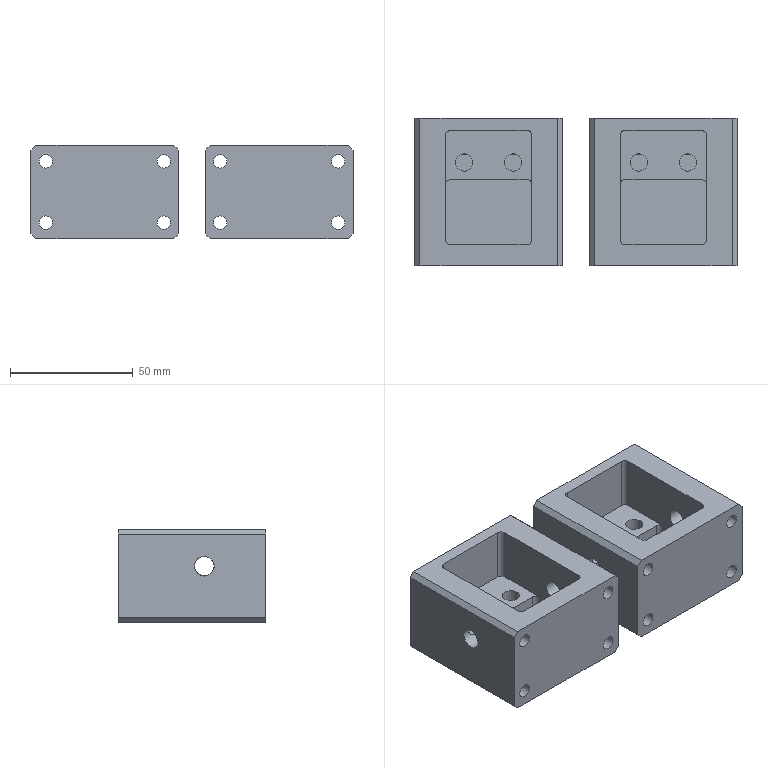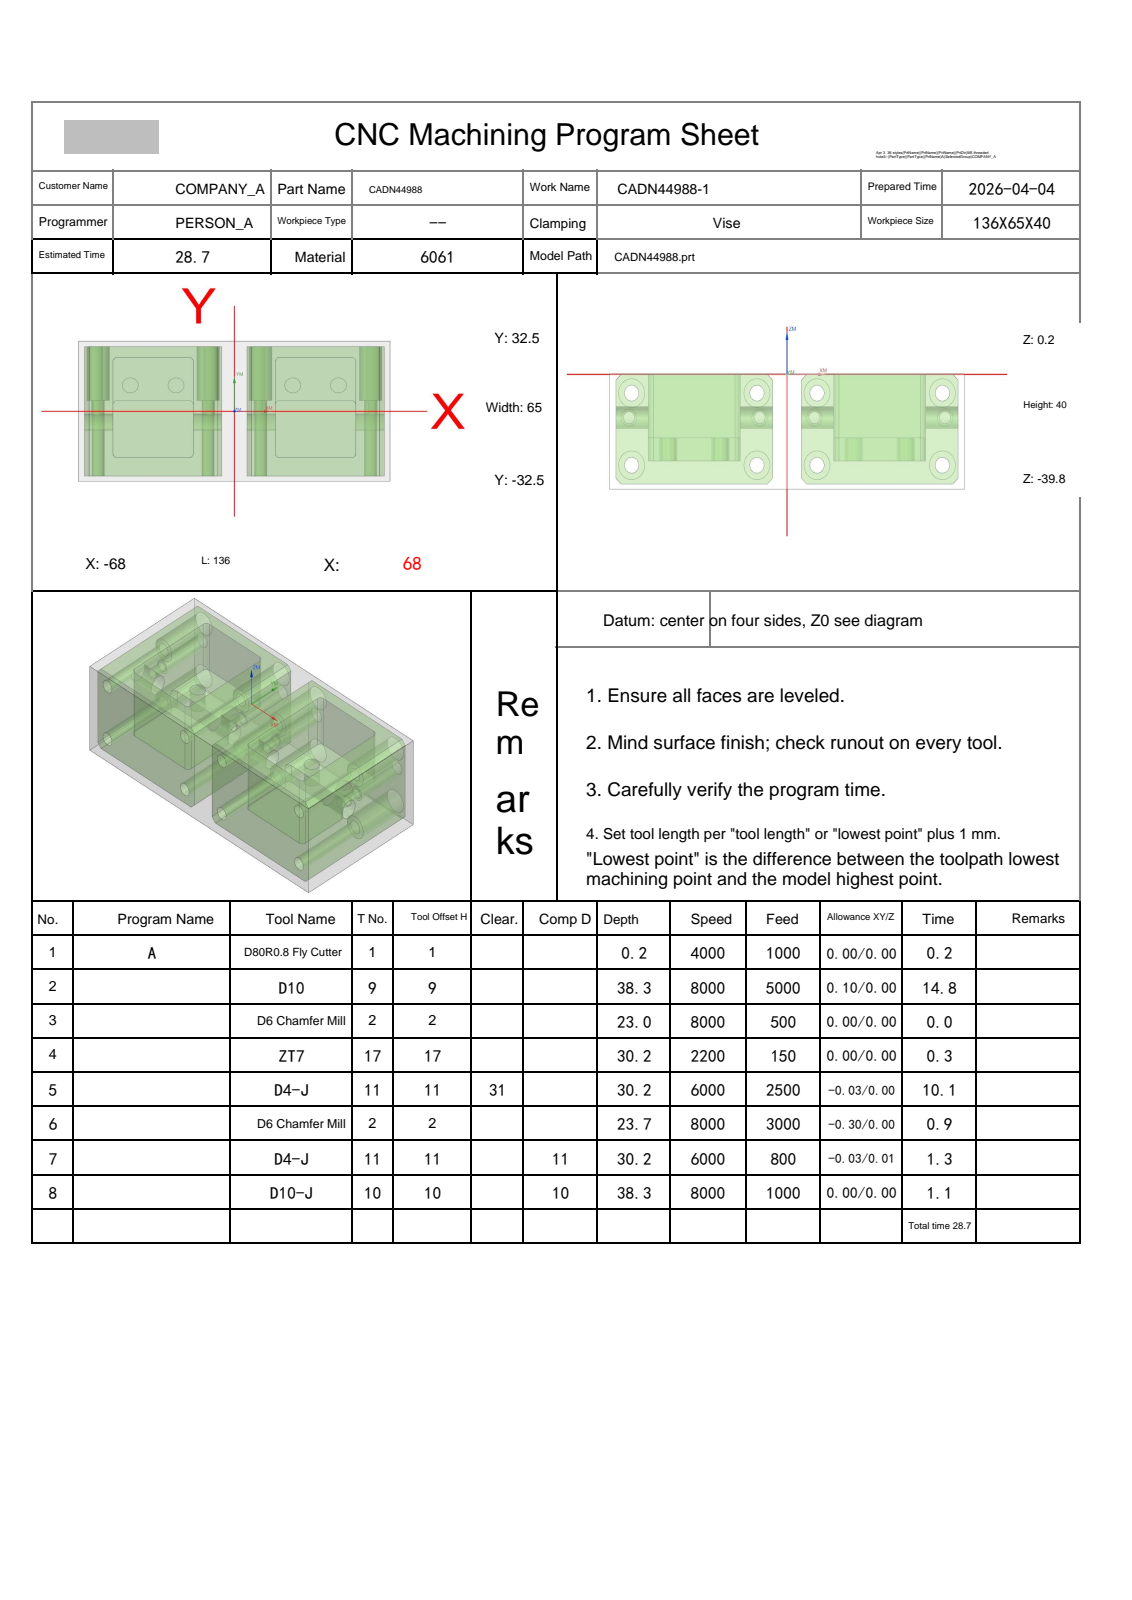NC program | NX | posted by the shop | part box 131 x 60 x 38 mm
Lines 33 to 1162 of 30516:
N2 T09 M06
(D10  D=10. R=0. H=09 ce=0.10 di=0.00)
G00 G90 G54 X35.5 Y-35.1 M03 S8000
G43 H09 Z20.
M08
Z.5
G01 X5.5 Z.413 F5000.
G02 X.4 Y-30. Z.39 I0.0 J5.1
G01 Y30. Z.216
G02 X5.5 Y35.1 Z.193 I5.1 J0.0
G01 X65.5 Z.019
G02 X70.6 Y30. Z-.004 I0.0 J-5.1
G01 Y-30. Z-.178
G02 X65.5 Y-35.1 Z-.201 I-5.1 J0.0
G01 X5.5 Z-.375
G02 X.4 Y-30. Z-.398 I0.0 J5.1
G01 Y30. Z-.572
G02 X5.5 Y35.1 Z-.595 I5.1 J0.0
G01 X65.5 Z-.769
G02 X70.6 Y30. Z-.792 I0.0 J-5.1
G01 Y-30. Z-.965
G02 X65.5 Y-35.1 Z-.989 I-5.1 J0.0
G01 X5.5 Z-1.162
G02 X.4 Y-30. Z-1.186 I0.0 J5.1
G01 Y30. Z-1.359
G02 X5.5 Y35.1 Z-1.383 I5.1 J0.0
G01 X65.5 Z-1.556
G02 X70.6 Y30. Z-1.579 I0.0 J-5.1
G01 Y-30. Z-1.753
G02 X65.5 Y-35.1 Z-1.776 I-5.1 J0.0
G01 X5.5 Z-1.95
G02 X.4 Y-30. Z-1.973 I0.0 J5.1
G01 Y30. Z-2.147
G02 X5.5 Y35.1 Z-2.17 I5.1 J0.0
G01 X65.5 Z-2.344
G02 X70.6 Y30. Z-2.367 I0.0 J-5.1
G01 Y-30. Z-2.541
G02 X65.5 Y-35.1 Z-2.564 I-5.1 J0.0
G01 X5.5 Z-2.738
G02 X.4 Y-30. Z-2.761 I0.0 J5.1
G01 Y30. Z-2.935
G02 X5.5 Y35.1 Z-2.958 I5.1 J0.0
G01 X65.5 Z-3.132
G02 X70.6 Y30. Z-3.155 I0.0 J-5.1
G01 Y-30. Z-3.329
G02 X65.5 Y-35.1 Z-3.352 I-5.1 J0.0
G01 X5.5 Z-3.526
G02 X.4 Y-30. Z-3.549 I0.0 J5.1
G01 Y30. Z-3.723
G02 X5.5 Y35.1 Z-3.746 I5.1 J0.0
G01 X65.5 Z-3.92
G02 X70.6 Y30. Z-3.943 I0.0 J-5.1
G01 Y-30. Z-4.116
G02 X65.5 Y-35.1 Z-4.14 I-5.1 J0.0
G01 X5.5 Z-4.313
G02 X.4 Y-30. Z-4.337 I0.0 J5.1
G01 Y30. Z-4.51
G02 X5.5 Y35.1 Z-4.534 I5.1 J0.0
G01 X65.5 Z-4.707
G02 X70.6 Y30. Z-4.73 I0.0 J-5.1
G01 Y-30. Z-4.904
G02 X65.5 Y-35.1 Z-4.927 I-5.1 J0.0
G01 X5.5 Z-5.101
G02 X.4 Y-30. Z-5.124 I0.0 J5.1
G01 Y30. Z-5.298
G02 X5.5 Y35.1 Z-5.321 I5.1 J0.0
G01 X65.5 Z-5.495
G02 X70.6 Y30. Z-5.518 I0.0 J-5.1
G01 Y-30. Z-5.692
G02 X65.5 Y-35.1 Z-5.715 I-5.1 J0.0
G01 X5.5 Z-5.889
G02 X.4 Y-30. Z-5.912 I0.0 J5.1
G01 Y30. Z-6.086
G02 X5.5 Y35.1 Z-6.109 I5.1 J0.0
G01 X65.5 Z-6.283
G02 X70.6 Y30. Z-6.306 I0.0 J-5.1
G01 Y-30. Z-6.48
G02 X65.5 Y-35.1 Z-6.503 I-5.1 J0.0
G01 X5.5 Z-6.677
G02 X.4 Y-30. Z-6.7 I0.0 J5.1
G01 Y30. Z-6.874
G02 X5.5 Y35.1 Z-6.897 I5.1 J0.0
G01 X65.5 Z-7.071
G02 X70.6 Y30. Z-7.094 I0.0 J-5.1
G01 Y-30. Z-7.267
G02 X65.5 Y-35.1 Z-7.291 I-5.1 J0.0
G01 X5.5 Z-7.464
G02 X.4 Y-30. Z-7.488 I0.0 J5.1
G01 Y30. Z-7.661
G02 X5.5 Y35.1 Z-7.685 I5.1 J0.0
G01 X65.5 Z-7.858
G02 X70.6 Y30. Z-7.881 I0.0 J-5.1
G01 Y-30. Z-8.055
G02 X65.5 Y-35.1 Z-8.078 I-5.1 J0.0
G01 X5.5 Z-8.252
G02 X.4 Y-30. Z-8.275 I0.0 J5.1
G01 Y30. Z-8.449
G02 X5.5 Y35.1 Z-8.472 I5.1 J0.0
G01 X65.5 Z-8.646
G02 X70.6 Y30. Z-8.669 I0.0 J-5.1
G01 Y-30. Z-8.843
G02 X65.5 Y-35.1 Z-8.866 I-5.1 J0.0
G01 X5.5 Z-9.04
G02 X.4 Y-30. Z-9.063 I0.0 J5.1
G01 Y30. Z-9.237
G02 X5.5 Y35.1 Z-9.26 I5.1 J0.0
G01 X65.5 Z-9.434
G02 X70.6 Y30. Z-9.457 I0.0 J-5.1
G01 Y-30. Z-9.631
G02 X65.5 Y-35.1 Z-9.654 I-5.1 J0.0
G01 X5.5 Z-9.828
G02 X.4 Y-30. Z-9.851 I0.0 J5.1
G01 Y30. Z-10.025
G02 X5.5 Y35.1 Z-10.048 I5.1 J0.0
G01 X65.5 Z-10.222
G02 X70.6 Y30. Z-10.245 I0.0 J-5.1
G01 Y-30. Z-10.419
G02 X65.5 Y-35.1 Z-10.442 I-5.1 J0.0
G01 X5.5 Z-10.615
G02 X.4 Y-30. Z-10.639 I0.0 J5.1
G01 Y30. Z-10.812
G02 X5.5 Y35.1 Z-10.836 I5.1 J0.0
G01 X65.5 Z-11.009
G02 X70.6 Y30. Z-11.033 I0.0 J-5.1
G01 Y-30. Z-11.206
G02 X65.5 Y-35.1 Z-11.229 I-5.1 J0.0
G01 X5.5 Z-11.403
G02 X.4 Y-30. Z-11.426 I0.0 J5.1
G01 Y30. Z-11.6
G02 X5.5 Y35.1 Z-11.623 I5.1 J0.0
G01 X65.5 Z-11.797
G02 X70.6 Y30. Z-11.82 I0.0 J-5.1
G01 Y-30. Z-11.994
G02 X65.5 Y-35.1 Z-12.017 I-5.1 J0.0
G01 X5.5 Z-12.191
G02 X.4 Y-30. Z-12.214 I0.0 J5.1
G01 Y30. Z-12.388
G02 X5.5 Y35.1 Z-12.411 I5.1 J0.0
G01 X65.5 Z-12.585
G02 X70.6 Y30. Z-12.608 I0.0 J-5.1
G01 Y-30. Z-12.782
G02 X65.5 Y-35.1 Z-12.805 I-5.1 J0.0
G01 X5.5 Z-12.979
G02 X.4 Y-30. Z-13.002 I0.0 J5.1
G01 Y30. Z-13.176
G02 X5.5 Y35.1 Z-13.199 I5.1 J0.0
G01 X65.5 Z-13.373
G02 X70.6 Y30. Z-13.396 I0.0 J-5.1
G01 Y-30. Z-13.57
G02 X65.5 Y-35.1 Z-13.593 I-5.1 J0.0
G01 X5.5 Z-13.766
G02 X.4 Y-30. Z-13.79 I0.0 J5.1
G01 Y30. Z-13.963
G02 X5.5 Y35.1 Z-13.987 I5.1 J0.0
G01 X65.5 Z-14.16
G02 X70.6 Y30. Z-14.184 I0.0 J-5.1
G01 Y-30. Z-14.357
G02 X65.5 Y-35.1 Z-14.38 I-5.1 J0.0
G01 X5.5 Z-14.554
G02 X.4 Y-30. Z-14.577 I0.0 J5.1
G01 Y30. Z-14.751
G02 X5.5 Y35.1 Z-14.774 I5.1 J0.0
G01 X65.5 Z-14.948
G02 X70.6 Y30. Z-14.971 I0.0 J-5.1
G01 Y-30. Z-15.145
G02 X65.5 Y-35.1 Z-15.168 I-5.1 J0.0
G01 X5.5 Z-15.342
G02 X.4 Y-30. Z-15.365 I0.0 J5.1
G01 Y30. Z-15.539
G02 X5.5 Y35.1 Z-15.562 I5.1 J0.0
G01 X65.5 Z-15.736
G02 X70.6 Y30. Z-15.759 I0.0 J-5.1
G01 Y-30. Z-15.933
G02 X65.5 Y-35.1 Z-15.956 I-5.1 J0.0
G01 X5.5 Z-16.13
G02 X.4 Y-30. Z-16.153 I0.0 J5.1
G01 Y30. Z-16.327
G02 X5.5 Y35.1 Z-16.35 I5.1 J0.0
G01 X65.5 Z-16.524
G02 X70.6 Y30. Z-16.547 I0.0 J-5.1
G01 Y-30. Z-16.721
G02 X65.5 Y-35.1 Z-16.744 I-5.1 J0.0
G01 X5.5 Z-16.917
G02 X.4 Y-30. Z-16.941 I0.0 J5.1
G01 Y30. Z-17.114
G02 X5.5 Y35.1 Z-17.138 I5.1 J0.0
G01 X65.5 Z-17.311
G02 X70.6 Y30. Z-17.335 I0.0 J-5.1
G01 Y-30. Z-17.508
G02 X65.5 Y-35.1 Z-17.531 I-5.1 J0.0
G01 X5.5 Z-17.705
G02 X.4 Y-30. Z-17.728 I0.0 J5.1
G01 Y30. Z-17.902
G02 X5.5 Y35.1 Z-17.925 I5.1 J0.0
G01 X65.5 Z-18.099
G02 X70.6 Y30. Z-18.122 I0.0 J-5.1
G01 Y-30. Z-18.296
G02 X65.5 Y-35.1 Z-18.319 I-5.1 J0.0
G01 X5.5 Z-18.493
G02 X.4 Y-30. Z-18.516 I0.0 J5.1
G01 Y30. Z-18.69
G02 X5.5 Y35.1 Z-18.713 I5.1 J0.0
G01 X65.5 Z-18.887
G02 X70.6 Y30. Z-18.91 I0.0 J-5.1
G01 Y-30. Z-19.084
G02 X65.5 Y-35.1 Z-19.107 I-5.1 J0.0
G01 X5.5 Z-19.281
G02 X.4 Y-30. Z-19.304 I0.0 J5.1
G01 Y30. Z-19.478
G02 X5.5 Y35.1 Z-19.501 I5.1 J0.0
G01 X65.5 Z-19.675
G02 X70.6 Y30. Z-19.698 I0.0 J-5.1
G01 Y-30. Z-19.872
G02 X65.5 Y-35.1 Z-19.895 I-5.1 J0.0
G01 X5.5 Z-20.069
G02 X.4 Y-30. Z-20.092 I0.0 J5.1
G01 Y30. Z-20.265
G02 X5.5 Y35.1 Z-20.289 I5.1 J0.0
G01 X65.5 Z-20.462
G02 X70.6 Y30. Z-20.486 I0.0 J-5.1
G01 Y-30. Z-20.659
G02 X65.5 Y-35.1 Z-20.683 I-5.1 J0.0
G01 X5.5 Z-20.856
G02 X.4 Y-30. Z-20.879 I0.0 J5.1
G01 Y30. Z-21.053
G02 X5.5 Y35.1 Z-21.076 I5.1 J0.0
G01 X65.5 Z-21.25
G02 X70.6 Y30. Z-21.273 I0.0 J-5.1
G01 Y-30. Z-21.447
G02 X65.5 Y-35.1 Z-21.47 I-5.1 J0.0
G01 X5.5 Z-21.644
G02 X.4 Y-30. Z-21.667 I0.0 J5.1
G01 Y30. Z-21.841
G02 X5.5 Y35.1 Z-21.864 I5.1 J0.0
G01 X65.5 Z-22.038
G02 X70.6 Y30. Z-22.061 I0.0 J-5.1
G01 Y-30. Z-22.235
G02 X65.5 Y-35.1 Z-22.258 I-5.1 J0.0
G01 X5.5 Z-22.432
G02 X.4 Y-30. Z-22.455 I0.0 J5.1
G01 Y30. Z-22.629
G02 X5.5 Y35.1 Z-22.652 I5.1 J0.0
G01 X65.5 Z-22.826
G02 X70.6 Y30. Z-22.849 I0.0 J-5.1
G01 Y-30. Z-23.023
G02 X65.5 Y-35.1 Z-23.046 I-5.1 J0.0
G01 X5.5 Z-23.22
G02 X.4 Y-30. Z-23.243 I0.0 J5.1
G01 Y30. Z-23.416
G02 X5.5 Y35.1 Z-23.44 I5.1 J0.0
G01 X65.5 Z-23.613
G02 X70.6 Y30. Z-23.637 I0.0 J-5.1
G01 Y-30. Z-23.81
G02 X65.5 Y-35.1 Z-23.834 I-5.1 J0.0
G01 X5.5 Z-24.007
G02 X.4 Y-30. Z-24.03 I0.0 J5.1
G01 Y30. Z-24.204
G02 X5.5 Y35.1 Z-24.227 I5.1 J0.0
G01 X65.5 Z-24.401
G02 X70.6 Y30. Z-24.424 I0.0 J-5.1
G01 Y-30. Z-24.598
G02 X65.5 Y-35.1 Z-24.621 I-5.1 J0.0
G01 X5.5 Z-24.795
G02 X.4 Y-30. Z-24.818 I0.0 J5.1
G01 Y30. Z-24.992
G02 X5.5 Y35.1 Z-25.015 I5.1 J0.0
G01 X65.5 Z-25.189
G02 X70.6 Y30. Z-25.212 I0.0 J-5.1
G01 Y-30. Z-25.386
G02 X65.5 Y-35.1 Z-25.409 I-5.1 J0.0
G01 X5.5 Z-25.583
G02 X.4 Y-30. Z-25.606 I0.0 J5.1
G01 Y30. Z-25.78
G02 X5.5 Y35.1 Z-25.803 I5.1 J0.0
G01 X65.5 Z-25.977
G02 X70.6 Y30. Z-26. I0.0 J-5.1
G01 Y-30. Z-26.174
G02 X65.5 Y-35.1 Z-26.197 I-5.1 J0.0
G01 X5.5 Z-26.371
G02 X.4 Y-30. Z-26.394 I0.0 J5.1
G01 Y30. Z-26.567
G02 X5.5 Y35.1 Z-26.591 I5.1 J0.0
G01 X65.5 Z-26.764
G02 X70.6 Y30. Z-26.788 I0.0 J-5.1
G01 Y-30. Z-26.961
G02 X65.5 Y-35.1 Z-26.985 I-5.1 J0.0
G01 X5.5 Z-27.158
G02 X.4 Y-30. Z-27.181 I0.0 J5.1
G01 Y30. Z-27.355
G02 X5.5 Y35.1 Z-27.378 I5.1 J0.0
G01 X65.5 Z-27.552
G02 X70.6 Y30. Z-27.575 I0.0 J-5.1
G01 Y-30. Z-27.749
G02 X65.5 Y-35.1 Z-27.772 I-5.1 J0.0
G01 X5.5 Z-27.946
G02 X.4 Y-30. Z-27.969 I0.0 J5.1
G01 Y30. Z-28.143
G02 X5.5 Y35.1 Z-28.166 I5.1 J0.0
G01 X65.5 Z-28.34
G02 X70.6 Y30. Z-28.363 I0.0 J-5.1
G01 Y-30. Z-28.537
G02 X65.5 Y-35.1 Z-28.56 I-5.1 J0.0
G01 X5.5 Z-28.734
G02 X.4 Y-30. Z-28.757 I0.0 J5.1
G01 Y30. Z-28.931
G02 X5.5 Y35.1 Z-28.954 I5.1 J0.0
G01 X65.5 Z-29.128
G02 X70.6 Y30. Z-29.151 I0.0 J-5.1
G01 Y-30. Z-29.325
G02 X65.5 Y-35.1 Z-29.348 I-5.1 J0.0
G01 X5.5 Z-29.522
G02 X.4 Y-30. Z-29.545 I0.0 J5.1
G01 Y30. Z-29.719
G02 X5.5 Y35.1 Z-29.742 I5.1 J0.0
G01 X65.5 Z-29.915
G02 X70.6 Y30. Z-29.939 I0.0 J-5.1
G01 Y-30. Z-30.112
G02 X65.5 Y-35.1 Z-30.136 I-5.1 J0.0
G01 X5.5 Z-30.309
G02 X.4 Y-30. Z-30.333 I0.0 J5.1
G01 Y30. Z-30.506
G02 X5.5 Y35.1 Z-30.529 I5.1 J0.0
G01 X65.5 Z-30.703
G02 X70.6 Y30. Z-30.726 I0.0 J-5.1
G01 Y-30. Z-30.9
G02 X65.5 Y-35.1 Z-30.923 I-5.1 J0.0
G01 X5.5 Z-31.097
G02 X.4 Y-30. Z-31.12 I0.0 J5.1
G01 Y30. Z-31.294
G02 X5.5 Y35.1 Z-31.317 I5.1 J0.0
G01 X65.5 Z-31.491
G02 X70.6 Y30. Z-31.514 I0.0 J-5.1
G01 Y-30. Z-31.688
G02 X65.5 Y-35.1 Z-31.711 I-5.1 J0.0
G01 X5.5 Z-31.885
G02 X.4 Y-30. Z-31.908 I0.0 J5.1
G01 Y30. Z-32.082
G02 X5.5 Y35.1 Z-32.105 I5.1 J0.0
G01 X65.5 Z-32.279
G02 X70.6 Y30. Z-32.302 I0.0 J-5.1
G01 Y-30. Z-32.476
G02 X65.5 Y-35.1 Z-32.499 I-5.1 J0.0
G01 X5.5 Z-32.673
G02 X.4 Y-30. Z-32.696 I0.0 J5.1
G01 Y30. Z-32.87
G02 X5.5 Y35.1 Z-32.893 I5.1 J0.0
G01 X65.5 Z-33.066
G02 X70.6 Y30. Z-33.09 I0.0 J-5.1
G01 Y-30. Z-33.263
G02 X65.5 Y-35.1 Z-33.287 I-5.1 J0.0
G01 X5.5 Z-33.46
G02 X.4 Y-30. Z-33.484 I0.0 J5.1
G01 Y30. Z-33.657
G02 X5.5 Y35.1 Z-33.68 I5.1 J0.0
G01 X65.5 Z-33.854
G02 X70.6 Y30. Z-33.877 I0.0 J-5.1
G01 Y-30. Z-34.051
G02 X65.5 Y-35.1 Z-34.074 I-5.1 J0.0
G01 X5.5 Z-34.248
G02 X.4 Y-30. Z-34.271 I0.0 J5.1
G01 Y30. Z-34.445
G02 X5.5 Y35.1 Z-34.468 I5.1 J0.0
G01 X65.5 Z-34.642
G02 X70.6 Y30. Z-34.665 I0.0 J-5.1
G01 Y-30. Z-34.839
G02 X65.5 Y-35.1 Z-34.862 I-5.1 J0.0
G01 X5.5 Z-35.036
G02 X.4 Y-30. Z-35.059 I0.0 J5.1
G01 Y30. Z-35.233
G02 X5.5 Y35.1 Z-35.256 I5.1 J0.0
G01 X65.5 Z-35.43
G02 X70.6 Y30. Z-35.453 I0.0 J-5.1
G01 Y-30. Z-35.627
G02 X65.5 Y-35.1 Z-35.65 I-5.1 J0.0
G01 X5.5 Z-35.824
G02 X.4 Y-30. Z-35.847 I0.0 J5.1
G01 Y30. Z-36.021
G02 X5.5 Y35.1 Z-36.044 I5.1 J0.0
G01 X65.5 Z-36.217
G02 X70.6 Y30. Z-36.241 I0.0 J-5.1
G01 Y-30. Z-36.414
G02 X65.5 Y-35.1 Z-36.438 I-5.1 J0.0
G01 X5.5 Z-36.611
G02 X.4 Y-30. Z-36.635 I0.0 J5.1
G01 Y30. Z-36.808
G02 X5.5 Y35.1 Z-36.831 I5.1 J0.0
G01 X65.5 Z-37.005
G02 X70.6 Y30. Z-37.028 I0.0 J-5.1
G01 Y-30. Z-37.202
G02 X65.5 Y-35.1 Z-37.225 I-5.1 J0.0
G01 X5.5 Z-37.399
G02 X.4 Y-30. Z-37.422 I0.0 J5.1
G01 Y30. Z-37.596
G02 X5.5 Y35.1 Z-37.619 I5.1 J0.0
G01 X65.5 Z-37.793
G02 X70.6 Y30. Z-37.816 I0.0 J-5.1
G01 Y-30. Z-37.99
G02 X65.5 Y-35.1 Z-38.013 I-5.1 J0.0
G01 X35.5 Z-38.1
X5.5
G02 X.4 Y-30. I0.0 J5.1
G01 Y30.
G02 X5.5 Y35.1 I5.1 J0.0
G01 X65.5
G02 X70.6 Y30. I0.0 J-5.1
G01 Y-30.
G02 X65.5 Y-35.1 I-5.1 J0.0
G01 X35.5
X35.
Z-37.1
G00 Z20.
X-35.5
Z.5
G01 X-65.5 Z.413
G02 X-70.6 Y-30. Z.39 I0.0 J5.1
G01 Y30. Z.216
G02 X-65.5 Y35.1 Z.193 I5.1 J0.0
G01 X-5.5 Z.019
G02 X-.4 Y30. Z-.004 I0.0 J-5.1
G01 Y-30. Z-.178
G02 X-5.5 Y-35.1 Z-.201 I-5.1 J0.0
G01 X-65.5 Z-.375
G02 X-70.6 Y-30. Z-.398 I0.0 J5.1
G01 Y30. Z-.572
G02 X-65.5 Y35.1 Z-.595 I5.1 J0.0
G01 X-5.5 Z-.769
G02 X-.4 Y30. Z-.792 I0.0 J-5.1
G01 Y-30. Z-.965
G02 X-5.5 Y-35.1 Z-.989 I-5.1 J0.0
G01 X-65.5 Z-1.162
G02 X-70.6 Y-30. Z-1.186 I0.0 J5.1
G01 Y30. Z-1.359
G02 X-65.5 Y35.1 Z-1.383 I5.1 J0.0
G01 X-5.5 Z-1.556
G02 X-.4 Y30. Z-1.579 I0.0 J-5.1
G01 Y-30. Z-1.753
G02 X-5.5 Y-35.1 Z-1.776 I-5.1 J0.0
G01 X-65.5 Z-1.95
G02 X-70.6 Y-30. Z-1.973 I0.0 J5.1
G01 Y30. Z-2.147
G02 X-65.5 Y35.1 Z-2.17 I5.1 J0.0
G01 X-5.5 Z-2.344
G02 X-.4 Y30. Z-2.367 I0.0 J-5.1
G01 Y-30. Z-2.541
G02 X-5.5 Y-35.1 Z-2.564 I-5.1 J0.0
G01 X-65.5 Z-2.738
G02 X-70.6 Y-30. Z-2.761 I0.0 J5.1
G01 Y30. Z-2.935
G02 X-65.5 Y35.1 Z-2.958 I5.1 J0.0
G01 X-5.5 Z-3.132
G02 X-.4 Y30. Z-3.155 I0.0 J-5.1
G01 Y-30. Z-3.329
G02 X-5.5 Y-35.1 Z-3.352 I-5.1 J0.0
G01 X-65.5 Z-3.526
G02 X-70.6 Y-30. Z-3.549 I0.0 J5.1
G01 Y30. Z-3.723
G02 X-65.5 Y35.1 Z-3.746 I5.1 J0.0
G01 X-5.5 Z-3.92
G02 X-.4 Y30. Z-3.943 I0.0 J-5.1
G01 Y-30. Z-4.116
G02 X-5.5 Y-35.1 Z-4.14 I-5.1 J0.0
G01 X-65.5 Z-4.313
G02 X-70.6 Y-30. Z-4.337 I0.0 J5.1
G01 Y30. Z-4.51
G02 X-65.5 Y35.1 Z-4.534 I5.1 J0.0
G01 X-5.5 Z-4.707
G02 X-.4 Y30. Z-4.73 I0.0 J-5.1
G01 Y-30. Z-4.904
G02 X-5.5 Y-35.1 Z-4.927 I-5.1 J0.0
G01 X-65.5 Z-5.101
G02 X-70.6 Y-30. Z-5.124 I0.0 J5.1
G01 Y30. Z-5.298
G02 X-65.5 Y35.1 Z-5.321 I5.1 J0.0
G01 X-5.5 Z-5.495
G02 X-.4 Y30. Z-5.518 I0.0 J-5.1
G01 Y-30. Z-5.692
G02 X-5.5 Y-35.1 Z-5.715 I-5.1 J0.0
G01 X-65.5 Z-5.889
G02 X-70.6 Y-30. Z-5.912 I0.0 J5.1
G01 Y30. Z-6.086
G02 X-65.5 Y35.1 Z-6.109 I5.1 J0.0
G01 X-5.5 Z-6.283
G02 X-.4 Y30. Z-6.306 I0.0 J-5.1
G01 Y-30. Z-6.48
G02 X-5.5 Y-35.1 Z-6.503 I-5.1 J0.0
G01 X-65.5 Z-6.677
G02 X-70.6 Y-30. Z-6.7 I0.0 J5.1
G01 Y30. Z-6.874
G02 X-65.5 Y35.1 Z-6.897 I5.1 J0.0
G01 X-5.5 Z-7.071
G02 X-.4 Y30. Z-7.094 I0.0 J-5.1
G01 Y-30. Z-7.267
G02 X-5.5 Y-35.1 Z-7.291 I-5.1 J0.0
G01 X-65.5 Z-7.464
G02 X-70.6 Y-30. Z-7.488 I0.0 J5.1
G01 Y30. Z-7.661
G02 X-65.5 Y35.1 Z-7.685 I5.1 J0.0
G01 X-5.5 Z-7.858
G02 X-.4 Y30. Z-7.881 I0.0 J-5.1
G01 Y-30. Z-8.055
G02 X-5.5 Y-35.1 Z-8.078 I-5.1 J0.0
G01 X-65.5 Z-8.252
G02 X-70.6 Y-30. Z-8.275 I0.0 J5.1
G01 Y30. Z-8.449
G02 X-65.5 Y35.1 Z-8.472 I5.1 J0.0
G01 X-5.5 Z-8.646
G02 X-.4 Y30. Z-8.669 I0.0 J-5.1
G01 Y-30. Z-8.843
G02 X-5.5 Y-35.1 Z-8.866 I-5.1 J0.0
G01 X-65.5 Z-9.04
G02 X-70.6 Y-30. Z-9.063 I0.0 J5.1
G01 Y30. Z-9.237
G02 X-65.5 Y35.1 Z-9.26 I5.1 J0.0
G01 X-5.5 Z-9.434
G02 X-.4 Y30. Z-9.457 I0.0 J-5.1
G01 Y-30. Z-9.631
G02 X-5.5 Y-35.1 Z-9.654 I-5.1 J0.0
G01 X-65.5 Z-9.828
G02 X-70.6 Y-30. Z-9.851 I0.0 J5.1
G01 Y30. Z-10.025
G02 X-65.5 Y35.1 Z-10.048 I5.1 J0.0
G01 X-5.5 Z-10.222
G02 X-.4 Y30. Z-10.245 I0.0 J-5.1
G01 Y-30. Z-10.419
G02 X-5.5 Y-35.1 Z-10.442 I-5.1 J0.0
G01 X-65.5 Z-10.615
G02 X-70.6 Y-30. Z-10.639 I0.0 J5.1
G01 Y30. Z-10.812
G02 X-65.5 Y35.1 Z-10.836 I5.1 J0.0
G01 X-5.5 Z-11.009
G02 X-.4 Y30. Z-11.033 I0.0 J-5.1
G01 Y-30. Z-11.206
G02 X-5.5 Y-35.1 Z-11.229 I-5.1 J0.0
G01 X-65.5 Z-11.403
G02 X-70.6 Y-30. Z-11.426 I0.0 J5.1
G01 Y30. Z-11.6
G02 X-65.5 Y35.1 Z-11.623 I5.1 J0.0
G01 X-5.5 Z-11.797
G02 X-.4 Y30. Z-11.82 I0.0 J-5.1
G01 Y-30. Z-11.994
G02 X-5.5 Y-35.1 Z-12.017 I-5.1 J0.0
G01 X-65.5 Z-12.191
G02 X-70.6 Y-30. Z-12.214 I0.0 J5.1
G01 Y30. Z-12.388
G02 X-65.5 Y35.1 Z-12.411 I5.1 J0.0
G01 X-5.5 Z-12.585
G02 X-.4 Y30. Z-12.608 I0.0 J-5.1
G01 Y-30. Z-12.782
G02 X-5.5 Y-35.1 Z-12.805 I-5.1 J0.0
G01 X-65.5 Z-12.979
G02 X-70.6 Y-30. Z-13.002 I0.0 J5.1
G01 Y30. Z-13.176
G02 X-65.5 Y35.1 Z-13.199 I5.1 J0.0
G01 X-5.5 Z-13.373
G02 X-.4 Y30. Z-13.396 I0.0 J-5.1
G01 Y-30. Z-13.57
G02 X-5.5 Y-35.1 Z-13.593 I-5.1 J0.0
G01 X-65.5 Z-13.766
G02 X-70.6 Y-30. Z-13.79 I0.0 J5.1
G01 Y30. Z-13.963
G02 X-65.5 Y35.1 Z-13.987 I5.1 J0.0
G01 X-5.5 Z-14.16
G02 X-.4 Y30. Z-14.184 I0.0 J-5.1
G01 Y-30. Z-14.357
G02 X-5.5 Y-35.1 Z-14.38 I-5.1 J0.0
G01 X-65.5 Z-14.554
G02 X-70.6 Y-30. Z-14.577 I0.0 J5.1
G01 Y30. Z-14.751
G02 X-65.5 Y35.1 Z-14.774 I5.1 J0.0
G01 X-5.5 Z-14.948
G02 X-.4 Y30. Z-14.971 I0.0 J-5.1
G01 Y-30. Z-15.145
G02 X-5.5 Y-35.1 Z-15.168 I-5.1 J0.0
G01 X-65.5 Z-15.342
G02 X-70.6 Y-30. Z-15.365 I0.0 J5.1
G01 Y30. Z-15.539
G02 X-65.5 Y35.1 Z-15.562 I5.1 J0.0
G01 X-5.5 Z-15.736
G02 X-.4 Y30. Z-15.759 I0.0 J-5.1
G01 Y-30. Z-15.933
G02 X-5.5 Y-35.1 Z-15.956 I-5.1 J0.0
G01 X-65.5 Z-16.13
G02 X-70.6 Y-30. Z-16.153 I0.0 J5.1
G01 Y30. Z-16.327
G02 X-65.5 Y35.1 Z-16.35 I5.1 J0.0
G01 X-5.5 Z-16.524
G02 X-.4 Y30. Z-16.547 I0.0 J-5.1
G01 Y-30. Z-16.721
G02 X-5.5 Y-35.1 Z-16.744 I-5.1 J0.0
G01 X-65.5 Z-16.917
G02 X-70.6 Y-30. Z-16.941 I0.0 J5.1
G01 Y30. Z-17.114
G02 X-65.5 Y35.1 Z-17.138 I5.1 J0.0
G01 X-5.5 Z-17.311
G02 X-.4 Y30. Z-17.335 I0.0 J-5.1
G01 Y-30. Z-17.508
G02 X-5.5 Y-35.1 Z-17.531 I-5.1 J0.0
G01 X-65.5 Z-17.705
G02 X-70.6 Y-30. Z-17.728 I0.0 J5.1
G01 Y30. Z-17.902
G02 X-65.5 Y35.1 Z-17.925 I5.1 J0.0
G01 X-5.5 Z-18.099
G02 X-.4 Y30. Z-18.122 I0.0 J-5.1
G01 Y-30. Z-18.296
G02 X-5.5 Y-35.1 Z-18.319 I-5.1 J0.0
G01 X-65.5 Z-18.493
G02 X-70.6 Y-30. Z-18.516 I0.0 J5.1
G01 Y30. Z-18.69
G02 X-65.5 Y35.1 Z-18.713 I5.1 J0.0
G01 X-5.5 Z-18.887
G02 X-.4 Y30. Z-18.91 I0.0 J-5.1
G01 Y-30. Z-19.084
G02 X-5.5 Y-35.1 Z-19.107 I-5.1 J0.0
G01 X-65.5 Z-19.281
G02 X-70.6 Y-30. Z-19.304 I0.0 J5.1
G01 Y30. Z-19.478
G02 X-65.5 Y35.1 Z-19.501 I5.1 J0.0
G01 X-5.5 Z-19.675
G02 X-.4 Y30. Z-19.698 I0.0 J-5.1
G01 Y-30. Z-19.872
G02 X-5.5 Y-35.1 Z-19.895 I-5.1 J0.0
G01 X-65.5 Z-20.069
G02 X-70.6 Y-30. Z-20.092 I0.0 J5.1
G01 Y30. Z-20.265
G02 X-65.5 Y35.1 Z-20.289 I5.1 J0.0
G01 X-5.5 Z-20.462
G02 X-.4 Y30. Z-20.486 I0.0 J-5.1
G01 Y-30. Z-20.659
G02 X-5.5 Y-35.1 Z-20.683 I-5.1 J0.0
G01 X-65.5 Z-20.856
G02 X-70.6 Y-30. Z-20.879 I0.0 J5.1
G01 Y30. Z-21.053
G02 X-65.5 Y35.1 Z-21.076 I5.1 J0.0
G01 X-5.5 Z-21.25
G02 X-.4 Y30. Z-21.273 I0.0 J-5.1
G01 Y-30. Z-21.447
G02 X-5.5 Y-35.1 Z-21.47 I-5.1 J0.0
G01 X-65.5 Z-21.644
G02 X-70.6 Y-30. Z-21.667 I0.0 J5.1
G01 Y30. Z-21.841
G02 X-65.5 Y35.1 Z-21.864 I5.1 J0.0
G01 X-5.5 Z-22.038
G02 X-.4 Y30. Z-22.061 I0.0 J-5.1
G01 Y-30. Z-22.235
G02 X-5.5 Y-35.1 Z-22.258 I-5.1 J0.0
G01 X-65.5 Z-22.432
G02 X-70.6 Y-30. Z-22.455 I0.0 J5.1
G01 Y30. Z-22.629
G02 X-65.5 Y35.1 Z-22.652 I5.1 J0.0
G01 X-5.5 Z-22.826
G02 X-.4 Y30. Z-22.849 I0.0 J-5.1
G01 Y-30. Z-23.023
G02 X-5.5 Y-35.1 Z-23.046 I-5.1 J0.0
G01 X-65.5 Z-23.22
G02 X-70.6 Y-30. Z-23.243 I0.0 J5.1
G01 Y30. Z-23.416
G02 X-65.5 Y35.1 Z-23.44 I5.1 J0.0
G01 X-5.5 Z-23.613
G02 X-.4 Y30. Z-23.637 I0.0 J-5.1
G01 Y-30. Z-23.81
G02 X-5.5 Y-35.1 Z-23.834 I-5.1 J0.0
G01 X-65.5 Z-24.007
G02 X-70.6 Y-30. Z-24.03 I0.0 J5.1
G01 Y30. Z-24.204
G02 X-65.5 Y35.1 Z-24.227 I5.1 J0.0
G01 X-5.5 Z-24.401
G02 X-.4 Y30. Z-24.424 I0.0 J-5.1
G01 Y-30. Z-24.598
G02 X-5.5 Y-35.1 Z-24.621 I-5.1 J0.0
G01 X-65.5 Z-24.795
G02 X-70.6 Y-30. Z-24.818 I0.0 J5.1
G01 Y30. Z-24.992
G02 X-65.5 Y35.1 Z-25.015 I5.1 J0.0
G01 X-5.5 Z-25.189
G02 X-.4 Y30. Z-25.212 I0.0 J-5.1
G01 Y-30. Z-25.386
G02 X-5.5 Y-35.1 Z-25.409 I-5.1 J0.0
G01 X-65.5 Z-25.583
G02 X-70.6 Y-30. Z-25.606 I0.0 J5.1
G01 Y30. Z-25.78
G02 X-65.5 Y35.1 Z-25.803 I5.1 J0.0
G01 X-5.5 Z-25.977
G02 X-.4 Y30. Z-26. I0.0 J-5.1
G01 Y-30. Z-26.174
G02 X-5.5 Y-35.1 Z-26.197 I-5.1 J0.0
G01 X-65.5 Z-26.371
G02 X-70.6 Y-30. Z-26.394 I0.0 J5.1
G01 Y30. Z-26.567
G02 X-65.5 Y35.1 Z-26.591 I5.1 J0.0
G01 X-5.5 Z-26.764
G02 X-.4 Y30. Z-26.788 I0.0 J-5.1
G01 Y-30. Z-26.961
G02 X-5.5 Y-35.1 Z-26.985 I-5.1 J0.0
G01 X-65.5 Z-27.158
G02 X-70.6 Y-30. Z-27.181 I0.0 J5.1
G01 Y30. Z-27.355
G02 X-65.5 Y35.1 Z-27.378 I5.1 J0.0
G01 X-5.5 Z-27.552
G02 X-.4 Y30. Z-27.575 I0.0 J-5.1
G01 Y-30. Z-27.749
G02 X-5.5 Y-35.1 Z-27.772 I-5.1 J0.0
G01 X-65.5 Z-27.946
G02 X-70.6 Y-30. Z-27.969 I0.0 J5.1
G01 Y30. Z-28.143
G02 X-65.5 Y35.1 Z-28.166 I5.1 J0.0
G01 X-5.5 Z-28.34
G02 X-.4 Y30. Z-28.363 I0.0 J-5.1
G01 Y-30. Z-28.537
G02 X-5.5 Y-35.1 Z-28.56 I-5.1 J0.0
G01 X-65.5 Z-28.734
G02 X-70.6 Y-30. Z-28.757 I0.0 J5.1
G01 Y30. Z-28.931
G02 X-65.5 Y35.1 Z-28.954 I5.1 J0.0
G01 X-5.5 Z-29.128
G02 X-.4 Y30. Z-29.151 I0.0 J-5.1
G01 Y-30. Z-29.325
G02 X-5.5 Y-35.1 Z-29.348 I-5.1 J0.0
G01 X-65.5 Z-29.522
G02 X-70.6 Y-30. Z-29.545 I0.0 J5.1
G01 Y30. Z-29.719
G02 X-65.5 Y35.1 Z-29.742 I5.1 J0.0
G01 X-5.5 Z-29.915
G02 X-.4 Y30. Z-29.939 I0.0 J-5.1
G01 Y-30. Z-30.112
G02 X-5.5 Y-35.1 Z-30.136 I-5.1 J0.0
G01 X-65.5 Z-30.309
G02 X-70.6 Y-30. Z-30.333 I0.0 J5.1
G01 Y30. Z-30.506
G02 X-65.5 Y35.1 Z-30.529 I5.1 J0.0
G01 X-5.5 Z-30.703
G02 X-.4 Y30. Z-30.726 I0.0 J-5.1
G01 Y-30. Z-30.9
G02 X-5.5 Y-35.1 Z-30.923 I-5.1 J0.0
G01 X-65.5 Z-31.097
G02 X-70.6 Y-30. Z-31.12 I0.0 J5.1
G01 Y30. Z-31.294
G02 X-65.5 Y35.1 Z-31.317 I5.1 J0.0
G01 X-5.5 Z-31.491
G02 X-.4 Y30. Z-31.514 I0.0 J-5.1
G01 Y-30. Z-31.688
G02 X-5.5 Y-35.1 Z-31.711 I-5.1 J0.0
G01 X-65.5 Z-31.885
G02 X-70.6 Y-30. Z-31.908 I0.0 J5.1
G01 Y30. Z-32.082
G02 X-65.5 Y35.1 Z-32.105 I5.1 J0.0
G01 X-5.5 Z-32.279
G02 X-.4 Y30. Z-32.302 I0.0 J-5.1
G01 Y-30. Z-32.476
G02 X-5.5 Y-35.1 Z-32.499 I-5.1 J0.0
G01 X-65.5 Z-32.673
G02 X-70.6 Y-30. Z-32.696 I0.0 J5.1
G01 Y30. Z-32.87
G02 X-65.5 Y35.1 Z-32.893 I5.1 J0.0
G01 X-5.5 Z-33.066
G02 X-.4 Y30. Z-33.09 I0.0 J-5.1
G01 Y-30. Z-33.263
G02 X-5.5 Y-35.1 Z-33.287 I-5.1 J0.0
G01 X-65.5 Z-33.46
G02 X-70.6 Y-30. Z-33.484 I0.0 J5.1
G01 Y30. Z-33.657
G02 X-65.5 Y35.1 Z-33.68 I5.1 J0.0
G01 X-5.5 Z-33.854
G02 X-.4 Y30. Z-33.877 I0.0 J-5.1
G01 Y-30. Z-34.051
G02 X-5.5 Y-35.1 Z-34.074 I-5.1 J0.0
G01 X-65.5 Z-34.248
G02 X-70.6 Y-30. Z-34.271 I0.0 J5.1
G01 Y30. Z-34.445
G02 X-65.5 Y35.1 Z-34.468 I5.1 J0.0
G01 X-5.5 Z-34.642
G02 X-.4 Y30. Z-34.665 I0.0 J-5.1
G01 Y-30. Z-34.839
G02 X-5.5 Y-35.1 Z-34.862 I-5.1 J0.0
G01 X-65.5 Z-35.036
G02 X-70.6 Y-30. Z-35.059 I0.0 J5.1
G01 Y30. Z-35.233
G02 X-65.5 Y35.1 Z-35.256 I5.1 J0.0
G01 X-5.5 Z-35.43
G02 X-.4 Y30. Z-35.453 I0.0 J-5.1
G01 Y-30. Z-35.627
G02 X-5.5 Y-35.1 Z-35.65 I-5.1 J0.0
G01 X-65.5 Z-35.824
G02 X-70.6 Y-30. Z-35.847 I0.0 J5.1
G01 Y30. Z-36.021
G02 X-65.5 Y35.1 Z-36.044 I5.1 J0.0
G01 X-5.5 Z-36.217
G02 X-.4 Y30. Z-36.241 I0.0 J-5.1
G01 Y-30. Z-36.414
G02 X-5.5 Y-35.1 Z-36.438 I-5.1 J0.0
G01 X-65.5 Z-36.611
G02 X-70.6 Y-30. Z-36.635 I0.0 J5.1
G01 Y30. Z-36.808
G02 X-65.5 Y35.1 Z-36.831 I5.1 J0.0
G01 X-5.5 Z-37.005
G02 X-.4 Y30. Z-37.028 I0.0 J-5.1
G01 Y-30. Z-37.202
G02 X-5.5 Y-35.1 Z-37.225 I-5.1 J0.0
G01 X-65.5 Z-37.399
G02 X-70.6 Y-30. Z-37.422 I0.0 J5.1
G01 Y30. Z-37.596
G02 X-65.5 Y35.1 Z-37.619 I5.1 J0.0
G01 X-5.5 Z-37.793
G02 X-.4 Y30. Z-37.816 I0.0 J-5.1
G01 Y-30. Z-37.99
G02 X-5.5 Y-35.1 Z-38.013 I-5.1 J0.0
G01 X-35.5 Z-38.1
X-65.5
G02 X-70.6 Y-30. I0.0 J5.1
G01 Y30.
G02 X-65.5 Y35.1 I5.1 J0.0
G01 X-5.5
G02 X-.4 Y30. I0.0 J-5.1
G01 Y-30.
G02 X-5.5 Y-35.1 I-5.1 J0.0
G01 X-35.5
X-36.
Z-37.1
G00 Z20.
G00 G90 X34.8 Y1.932 M03 S6000
Z20.
Z.7
M03 S6000
G01 Y-4.6 Z.472 F2800.
X36.2 Z.423
Y8.1 Z-.02
X34.8 Z-.069
Y1.75 Z-.291
X34.5
M03 S6000
Y-4.9 F3500.
X36.5
Y8.4
X34.5
Y1.75
X30.
Y-9.4
X41.
Y12.9
X30.
Y1.75
X23.
Y-16.4
X48.
Y19.9
X23.
Y1.75
Z.709
G00 Z1.2
X34.8 Y1.932
Z.209
M03 S6000
G01 Y-4.6 Z-.019 F2800.
X36.2 Z-.068
Y8.1 Z-.512
X34.8 Z-.56
Y1.75 Z-.782
X34.5
M03 S6000
Y-4.9 F3500.
X36.5
Y8.4
X34.5
Y1.75
X30.
Y-9.4
X41.
Y12.9
X30.
Y1.75
X23.
Y-16.4
X48.
Y19.9
X23.
Y1.75
Z.218
G00 Z.709
X34.8 Y1.932
Z-.282
M03 S6000
G01 Y-4.6 Z-.51 F2800.
X36.2 Z-.559
Y8.1 Z-1.003
X34.8 Z-1.052
Y1.75 Z-1.273
X34.5
M03 S6000
Y-4.9 F3500.
X36.5
Y8.4
X34.5
Y1.75
X30.
Y-9.4
X41.
Y12.9
X30.
Y1.75
X23.
Y-16.4
X48.
Y19.9
X23.
Y1.75
Z-.273
G00 Z.218
X34.8 Y1.932
Z-.773
M03 S6000
G01 Y-4.6 Z-1.001 F2800.
X36.2 Z-1.05
Y8.1 Z-1.494
X34.8 Z-1.543
Y1.75 Z-1.764
X34.5
M03 S6000
Y-4.9 F3500.
X36.5
Y8.4
X34.5
Y1.75
X30.
Y-9.4
X41.
Y12.9
X30.
Y1.75
X23.
Y-16.4
X48.
Y19.9
X23.
Y1.75
Z-.764
G00 Z-.273
X34.8 Y1.932
Z-1.264
M03 S6000
G01 Y-4.6 Z-1.493 F2800.
X36.2 Z-1.541
Y8.1 Z-1.985
X34.8 Z-2.034
Y1.75 Z-2.256
X34.5
M03 S6000
Y-4.9 F3500.
X36.5
Y8.4
X34.5
Y1.75
X30.
Y-9.4
X41.
Y12.9
X30.
Y1.75
X23.
Y-16.4
X48.
Y19.9
X23.
Y1.75
Z-1.256
G00 Z-.764
X34.8 Y1.932
Z-1.756
M03 S6000
G01 Y-4.6 Z-1.984 F2800.
X36.2 Z-2.033
Y8.1 Z-2.476
X34.8 Z-2.525
Y1.75 Z-2.747
X34.5
M03 S6000
Y-4.9 F3500.
X36.5
Y8.4
X34.5
Y1.75
X30.
Y-9.4
X41.
Y12.9
X30.
Y1.75
X23.
Y-16.4
X48.
Y19.9
X23.
Y1.75
Z-1.747
G00 Z-1.256
X34.8 Y1.932
Z-2.247
M03 S6000
G01 Y-4.6 Z-2.475 F2800.
X36.2 Z-2.524
Y8.1 Z-2.967
X34.8 Z-3.016
Y1.75 Z-3.238
X34.5
M03 S6000
Y-4.9 F3500.
X36.5
Y8.4
X34.5
Y1.75
X30.
Y-9.4
X41.
Y12.9
X30.
Y1.75
X23.
Y-16.4
X48.
Y19.9
X23.
Y1.75
Z-2.238
G00 Z-1.747
X34.8 Y1.932
Z-2.738
M03 S6000
G01 Y-4.6 Z-2.966 F2800.
X36.2 Z-3.015
Y8.1 Z-3.458
X34.8 Z-3.507
Y1.75 Z-3.729
X34.5
M03 S6000
Y-4.9 F3500.
X36.5
Y8.4
X34.5
Y1.75
X30.
Y-9.4
X41.
Y12.9
X30.
Y1.75
X23.
Y-16.4
X48.
Y19.9
X23.
Y1.75
Z-2.729
G00 Z-2.238
X34.8 Y1.932
Z-3.229
M03 S6000
G01 Y-4.6 Z-3.457 F2800.
X36.2 Z-3.506
Y8.1 Z-3.949
X34.8 Z-3.998
Y1.75 Z-4.22
X34.5
M03 S6000
Y-4.9 F3500.
X36.5
Y8.4
X34.5
Y1.75
X30.
Y-9.4
X41.
Y12.9
X30.
Y1.75
X23.
Y-16.4
X48.
Y19.9
X23.
Y1.75
Z-3.22
G00 Z-2.729
X34.8 Y1.932
Z-3.72
M03 S6000
G01 Y-4.6 Z-3.948 F2800.
X36.2 Z-3.997
Y8.1 Z-4.44
X34.8 Z-4.489
Y1.75 Z-4.711
X34.5
M03 S6000
Y-4.9 F3500.
X36.5
Y8.4
X34.5
Y1.75
X30.
Y-9.4
X41.
Y12.9
X30.
Y1.75
X23.
Y-16.4
X48.
Y19.9
X23.
Y1.75
Z-3.711
G00 Z-3.22
X34.8 Y1.932
Z-4.211
M03 S6000
G01 Y-4.6 Z-4.439 F2800.
X36.2 Z-4.488
Y8.1 Z-4.932
X34.8 Z-4.98
Y1.75 Z-5.202
X34.5
M03 S6000
Y-4.9 F3500.
X36.5
Y8.4
X34.5
Y1.75
X30.
Y-9.4
X41.
Y12.9
X30.
Y1.75